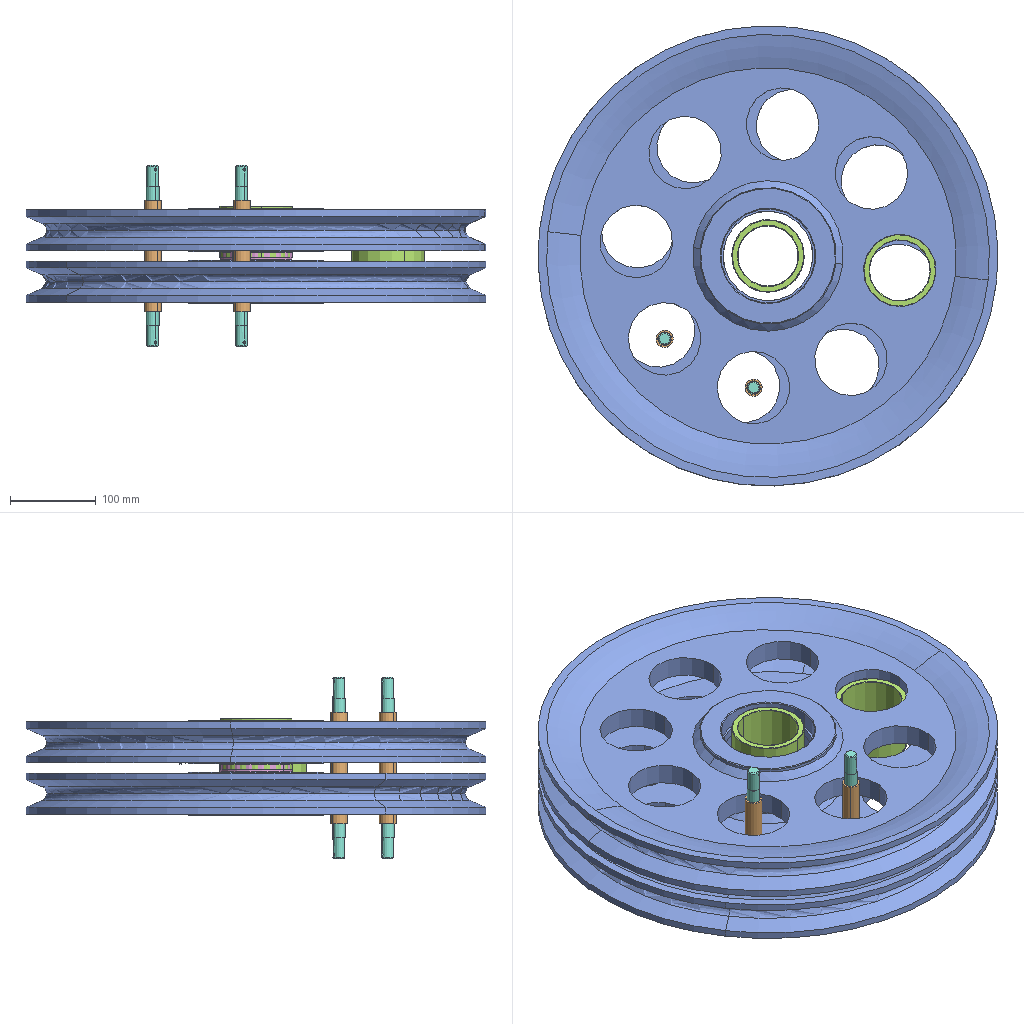Assembly | SolidWorks | 6 different items | 11 placed | box 538 x 538 x 212 mm
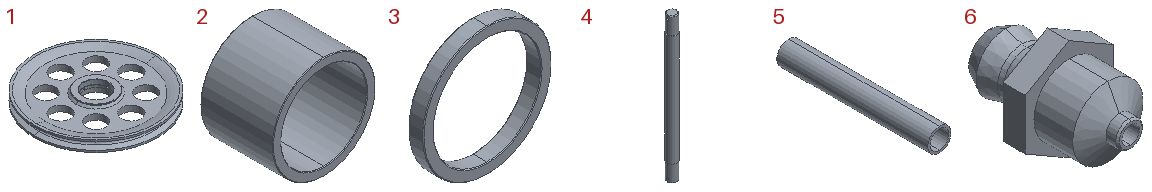Parts list (item | quantity | size | volume | features):
1 | x2 | 538 x 538 x 50 mm | 4931850 mm3 | features ICE 3, Revolution 2, Chamfer 1, CirPattern 1, CombineBodies 1
2 | x2 | 85 x 60 x 85 mm | 102796 mm3 | features Chamfer 1, Extrusion 1
3 | x1 | 85 x 10 x 85 mm | 17031 mm3 | features Chamfer 1, Extrusion 1
4 | x2 | 15 x 15 x 212 mm | 36086 mm3 | features Chamfer 1, ICE 1, Revolution 1
5 | x2 | 20 x 130 x 20 mm | 14703 mm3 | features Extrusion 1
6 | x2 | 10 x 16 x 11.547 mm | 627.343 mm3 | features Boss 1, Chamfer 1, Revolution 1
Mates (type | each side: item.copy, entity, surface, feature):
Concentric | 4.1 face cylinder Revolve1 | 5.1 face cylinder Boss-Extrude1
Width | 5.1 face plane Boss-Extrude1 | 5.1 face plane Boss-Extrude1 | 4.1 face plane Revolve1 | 4.1 face plane Revolve1
Concentric | 4.2 face cylinder Revolve1 | 5.2 face cylinder Boss-Extrude1
Width | 5.2 face plane Boss-Extrude1 | 5.2 face plane Boss-Extrude1 | 4.2 face plane Revolve1 | 4.2 face plane Revolve1
Concentric | 1.1 face cylinder Combine1 | 6.1 face cylinder Revolve2
Concentric | 1.2 face cylinder Combine1 | 6.2 face cylinder Revolve2
Parallel | 1.1 face cylinder CirPattern1 | 5.1 face cylinder Boss-Extrude1
Concentric | 1.1 face cylinder Revolve1 | 2.1 face cylinder Boss-Extrude1
Coincident | 1.1 edge | 2.2 face cylinder Boss-Extrude1
Parallel | 1.1 face cylinder CirPattern1 | 5.2 face cylinder Boss-Extrude1
Concentric | 1.1 face cylinder CirPattern1 | 5.1 face cylinder Boss-Extrude1
Concentric | 1.1 face cylinder CirPattern1 | 5.2 face cylinder Boss-Extrude1